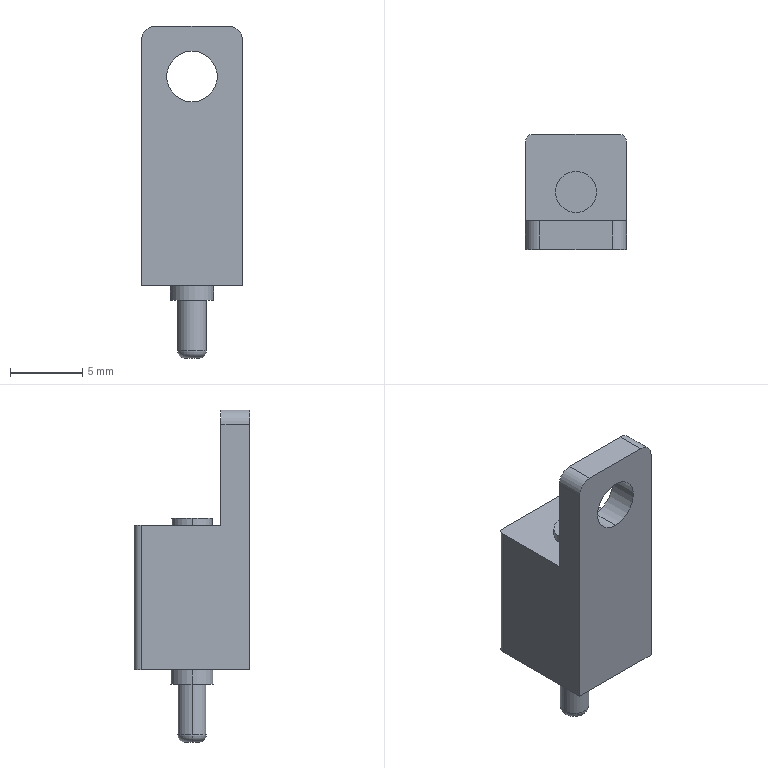Part | SolidWorks | features ICE 5, Fillet 3, Extrusion 1 | 1 solid | 25 faces | box 7 x 8 x 23 mm | volume 673.267 mm3 | cylinder 12 | plane 11 | torus 2 | commonest cylinder face diameters 2 x4 1 x2 2.853 x2 2.98 x2 3.5 x2
STEP:
#1=CARTESIAN_POINT('',(0.,-4.,12.75));
#2=VERTEX_POINT('',#1);
#3=CARTESIAN_POINT('',(0.,-4.,16.25));
#4=VERTEX_POINT('',#3);
#5=CARTESIAN_POINT('',(0.,-4.,14.5));
#6=DIRECTION('',(0.,1.,0.));
#7=DIRECTION('',(0.,0.,1.));
#8=AXIS2_PLACEMENT_3D('',#5,#6,#7);
#9=CIRCLE('',#8,1.75);
#10=EDGE_CURVE('',#2,#4,#9,.T.);
#11=ORIENTED_EDGE('',*,*,#10,.F.);
#12=CARTESIAN_POINT('',(0.,-2.,12.75));
#13=VERTEX_POINT('',#12);
#14=CARTESIAN_POINT('',(0.,-4.,12.75));
#15=DIRECTION('',(0.,1.,0.));
#16=VECTOR('',#15,1000.);
#17=LINE('',#14,#16);
#18=EDGE_CURVE('',#2,#13,#17,.T.);
#19=ORIENTED_EDGE('',*,*,#18,.T.);
#20=CARTESIAN_POINT('',(0.,-2.,16.25));
#21=VERTEX_POINT('',#20);
#22=CARTESIAN_POINT('',(0.,-2.,14.5));
#23=DIRECTION('',(0.,1.,0.));
#24=DIRECTION('',(0.,0.,1.));
#25=AXIS2_PLACEMENT_3D('',#22,#23,#24);
#26=CIRCLE('',#25,1.75);
#27=EDGE_CURVE('',#13,#21,#26,.T.);
#28=ORIENTED_EDGE('',*,*,#27,.T.);
#29=CARTESIAN_POINT('',(0.,-4.,16.25));
#30=DIRECTION('',(0.,1.,0.));
#31=VECTOR('',#30,1000.);
#32=LINE('',#29,#31);
#33=EDGE_CURVE('',#4,#21,#32,.T.);
#34=ORIENTED_EDGE('',*,*,#33,.F.);
#35=EDGE_LOOP('',(#11,#19,#28,#34));
#36=FACE_OUTER_BOUND('',#35,.T.);
#37=CARTESIAN_POINT('',(0.,-4.,14.5));
#38=DIRECTION('',(0.,1.,0.));
#39=DIRECTION('',(0.,0.,1.));
#40=AXIS2_PLACEMENT_3D('',#37,#38,#39);
#41=CYLINDRICAL_SURFACE('',#40,1.75);
#42=ADVANCED_FACE('',(#36),#41,.F.);
#43=CARTESIAN_POINT('',(1.427,0.,10.5));
#44=VERTEX_POINT('',#43);
#45=CARTESIAN_POINT('',(-1.427,0.,10.5));
#46=VERTEX_POINT('',#45);
#47=CARTESIAN_POINT('',(0.,0.,10.5));
#48=DIRECTION('',(0.,0.,1.));
#49=DIRECTION('',(1.,0.,0.));
#50=AXIS2_PLACEMENT_3D('',#47,#48,#49);
#51=CIRCLE('',#50,1.427);
#52=EDGE_CURVE('',#44,#46,#51,.T.);
#53=ORIENTED_EDGE('',*,*,#52,.F.);
#54=CARTESIAN_POINT('',(1.427,0.,10.));
#55=VERTEX_POINT('',#54);
#56=CARTESIAN_POINT('',(1.427,0.,10.5));
#57=DIRECTION('',(0.,0.,-1.));
#58=VECTOR('',#57,1000.);
#59=LINE('',#56,#58);
#60=EDGE_CURVE('',#44,#55,#59,.T.);
#61=ORIENTED_EDGE('',*,*,#60,.T.);
#62=CARTESIAN_POINT('',(-1.427,0.,10.));
#63=VERTEX_POINT('',#62);
#64=CARTESIAN_POINT('',(0.,0.,10.));
#65=DIRECTION('',(0.,0.,1.));
#66=DIRECTION('',(1.,0.,0.));
#67=AXIS2_PLACEMENT_3D('',#64,#65,#66);
#68=CIRCLE('',#67,1.427);
#69=EDGE_CURVE('',#55,#63,#68,.T.);
#70=ORIENTED_EDGE('',*,*,#69,.T.);
#71=CARTESIAN_POINT('',(-1.427,0.,10.5));
#72=DIRECTION('',(0.,0.,-1.));
#73=VECTOR('',#72,1000.);
#74=LINE('',#71,#73);
#75=EDGE_CURVE('',#46,#63,#74,.T.);
#76=ORIENTED_EDGE('',*,*,#75,.F.);
#77=EDGE_LOOP('',(#53,#61,#70,#76));
#78=FACE_OUTER_BOUND('',#77,.T.);
#79=CARTESIAN_POINT('',(0.,0.,10.5));
#80=DIRECTION('',(0.,0.,-1.));
#81=DIRECTION('',(-1.,0.,0.));
#82=AXIS2_PLACEMENT_3D('',#79,#80,#81);
#83=CYLINDRICAL_SURFACE('',#82,1.427);
#84=ADVANCED_FACE('',(#78),#83,.T.);
#85=CARTESIAN_POINT('',(1.,0.,-4.5));
#86=VERTEX_POINT('',#85);
#87=CARTESIAN_POINT('',(-1.,0.,-4.5));
#88=VERTEX_POINT('',#87);
#89=CARTESIAN_POINT('',(0.,0.,-4.5));
#90=DIRECTION('',(0.,0.,1.));
#91=DIRECTION('',(-1.,0.,0.));
#92=AXIS2_PLACEMENT_3D('',#89,#90,#91);
#93=CIRCLE('',#92,1.);
#94=EDGE_CURVE('',#86,#88,#93,.T.);
#95=ORIENTED_EDGE('',*,*,#94,.T.);
#96=CARTESIAN_POINT('',(-1.,0.,-1.));
#97=VERTEX_POINT('',#96);
#98=CARTESIAN_POINT('',(-1.,0.,-5.));
#99=DIRECTION('',(0.,0.,1.));
#100=VECTOR('',#99,1000.);
#101=LINE('',#98,#100);
#102=EDGE_CURVE('',#88,#97,#101,.T.);
#103=ORIENTED_EDGE('',*,*,#102,.T.);
#104=CARTESIAN_POINT('',(1.,0.,-1.));
#105=VERTEX_POINT('',#104);
#106=CARTESIAN_POINT('',(0.,0.,-1.));
#107=DIRECTION('',(0.,0.,-1.));
#108=DIRECTION('',(-1.,0.,0.));
#109=AXIS2_PLACEMENT_3D('',#106,#107,#108);
#110=CIRCLE('',#109,1.);
#111=EDGE_CURVE('',#97,#105,#110,.T.);
#112=ORIENTED_EDGE('',*,*,#111,.T.);
#113=CARTESIAN_POINT('',(1.,0.,-5.));
#114=DIRECTION('',(0.,0.,1.));
#115=VECTOR('',#114,1000.);
#116=LINE('',#113,#115);
#117=EDGE_CURVE('',#86,#105,#116,.T.);
#118=ORIENTED_EDGE('',*,*,#117,.F.);
#119=EDGE_LOOP('',(#95,#103,#112,#118));
#120=FACE_OUTER_BOUND('',#119,.T.);
#121=CARTESIAN_POINT('',(0.,0.,-5.));
#122=DIRECTION('',(0.,0.,1.));
#123=DIRECTION('',(1.,0.,0.));
#124=AXIS2_PLACEMENT_3D('',#121,#122,#123);
#125=CYLINDRICAL_SURFACE('',#124,1.);
#126=ADVANCED_FACE('',(#120),#125,.T.);
#127=ORIENTED_EDGE('',*,*,#94,.F.);
#128=CARTESIAN_POINT('',(0.5,0.,-5.));
#129=VERTEX_POINT('',#128);
#130=CARTESIAN_POINT('',(0.5,0.,-4.5));
#131=DIRECTION('',(0.,1.,0.));
#132=DIRECTION('',(-1.,0.,0.));
#133=AXIS2_PLACEMENT_3D('',#130,#131,#132);
#134=CIRCLE('',#133,0.5);
#135=EDGE_CURVE('',#86,#129,#134,.T.);
#136=ORIENTED_EDGE('',*,*,#135,.T.);
#137=CARTESIAN_POINT('',(-0.5,0.,-5.));
#138=VERTEX_POINT('',#137);
#139=CARTESIAN_POINT('',(0.,0.,-5.));
#140=DIRECTION('',(0.,0.,-1.));
#141=DIRECTION('',(-1.,0.,0.));
#142=AXIS2_PLACEMENT_3D('',#139,#140,#141);
#143=CIRCLE('',#142,0.5);
#144=EDGE_CURVE('',#138,#129,#143,.T.);
#145=ORIENTED_EDGE('',*,*,#144,.F.);
#146=CARTESIAN_POINT('',(-0.5,0.,-4.5));
#147=DIRECTION('',(0.,-1.,0.));
#148=DIRECTION('',(0.,0.,-1.));
#149=AXIS2_PLACEMENT_3D('',#146,#147,#148);
#150=CIRCLE('',#149,0.5);
#151=EDGE_CURVE('',#88,#138,#150,.T.);
#152=ORIENTED_EDGE('',*,*,#151,.F.);
#153=EDGE_LOOP('',(#127,#136,#145,#152));
#154=FACE_OUTER_BOUND('',#153,.T.);
#155=CARTESIAN_POINT('',(0.,0.,-4.5));
#156=DIRECTION('',(0.,0.,-1.));
#157=DIRECTION('',(-1.,0.,0.));
#158=AXIS2_PLACEMENT_3D('',#155,#156,#157);
#159=TOROIDAL_SURFACE('',#158,0.5,0.5);
#160=ADVANCED_FACE('',(#154),#159,.T.);
#161=CARTESIAN_POINT('',(-1.49,0.,-1.));
#162=VERTEX_POINT('',#161);
#163=CARTESIAN_POINT('',(1.49,0.,-1.));
#164=VERTEX_POINT('',#163);
#165=CARTESIAN_POINT('',(0.,0.,-1.));
#166=DIRECTION('',(0.,0.,-1.));
#167=DIRECTION('',(-1.,0.,0.));
#168=AXIS2_PLACEMENT_3D('',#165,#166,#167);
#169=CIRCLE('',#168,1.49);
#170=EDGE_CURVE('',#162,#164,#169,.T.);
#171=ORIENTED_EDGE('',*,*,#170,.F.);
#172=CARTESIAN_POINT('',(-1.49,0.,0.));
#173=VERTEX_POINT('',#172);
#174=CARTESIAN_POINT('',(-1.49,0.,-1.));
#175=DIRECTION('',(0.,0.,1.));
#176=VECTOR('',#175,1000.);
#177=LINE('',#174,#176);
#178=EDGE_CURVE('',#162,#173,#177,.T.);
#179=ORIENTED_EDGE('',*,*,#178,.T.);
#180=CARTESIAN_POINT('',(1.49,0.,0.));
#181=VERTEX_POINT('',#180);
#182=CARTESIAN_POINT('',(0.,0.,0.));
#183=DIRECTION('',(0.,0.,-1.));
#184=DIRECTION('',(1.,0.,0.));
#185=AXIS2_PLACEMENT_3D('',#182,#183,#184);
#186=CIRCLE('',#185,1.49);
#187=EDGE_CURVE('',#173,#181,#186,.T.);
#188=ORIENTED_EDGE('',*,*,#187,.T.);
#189=CARTESIAN_POINT('',(1.49,0.,-1.));
#190=DIRECTION('',(0.,0.,1.));
#191=VECTOR('',#190,1000.);
#192=LINE('',#189,#191);
#193=EDGE_CURVE('',#164,#181,#192,.T.);
#194=ORIENTED_EDGE('',*,*,#193,.F.);
#195=EDGE_LOOP('',(#171,#179,#188,#194));
#196=FACE_OUTER_BOUND('',#195,.T.);
#197=CARTESIAN_POINT('',(0.,0.,-1.));
#198=DIRECTION('',(0.,0.,1.));
#199=DIRECTION('',(1.,0.,0.));
#200=AXIS2_PLACEMENT_3D('',#197,#198,#199);
#201=CYLINDRICAL_SURFACE('',#200,1.49);
#202=ADVANCED_FACE('',(#196),#201,.T.);
#203=CARTESIAN_POINT('',(3.5,-2.,17.));
#204=VERTEX_POINT('',#203);
#205=CARTESIAN_POINT('',(3.5,-2.,10.));
#206=VERTEX_POINT('',#205);
#207=CARTESIAN_POINT('',(3.5,-2.,18.));
#208=DIRECTION('',(0.,0.,-1.));
#209=VECTOR('',#208,1000.);
#210=LINE('',#207,#209);
#211=EDGE_CURVE('',#204,#206,#210,.T.);
#212=ORIENTED_EDGE('',*,*,#211,.F.);
#213=CARTESIAN_POINT('',(3.5,-4.,17.));
#214=VERTEX_POINT('',#213);
#215=CARTESIAN_POINT('',(3.5,-4.,17.));
#216=DIRECTION('',(0.,-1.,0.));
#217=VECTOR('',#216,1000.);
#218=LINE('',#215,#217);
#219=EDGE_CURVE('',#204,#214,#218,.T.);
#220=ORIENTED_EDGE('',*,*,#219,.T.);
#221=CARTESIAN_POINT('',(3.5,-4.,0.));
#222=VERTEX_POINT('',#221);
#223=CARTESIAN_POINT('',(3.5,-4.,10.));
#224=DIRECTION('',(0.,0.,-1.));
#225=VECTOR('',#224,1000.);
#226=LINE('',#223,#225);
#227=EDGE_CURVE('',#214,#222,#226,.T.);
#228=ORIENTED_EDGE('',*,*,#227,.T.);
#229=CARTESIAN_POINT('',(3.5,3.5,0.));
#230=VERTEX_POINT('',#229);
#231=CARTESIAN_POINT('',(3.5,4.,0.));
#232=DIRECTION('',(0.,1.,0.));
#233=VECTOR('',#232,1000.);
#234=LINE('',#231,#233);
#235=EDGE_CURVE('',#222,#230,#234,.T.);
#236=ORIENTED_EDGE('',*,*,#235,.T.);
#237=CARTESIAN_POINT('',(3.5,3.5,10.));
#238=VERTEX_POINT('',#237);
#239=CARTESIAN_POINT('',(3.5,3.5,10.));
#240=DIRECTION('',(0.,0.,1.));
#241=VECTOR('',#240,1000.);
#242=LINE('',#239,#241);
#243=EDGE_CURVE('',#230,#238,#242,.T.);
#244=ORIENTED_EDGE('',*,*,#243,.T.);
#245=CARTESIAN_POINT('',(3.5,4.,10.));
#246=DIRECTION('',(0.,1.,0.));
#247=VECTOR('',#246,1000.);
#248=LINE('',#245,#247);
#249=EDGE_CURVE('',#206,#238,#248,.T.);
#250=ORIENTED_EDGE('',*,*,#249,.F.);
#251=EDGE_LOOP('',(#212,#220,#228,#236,#244,#250));
#252=FACE_OUTER_BOUND('',#251,.T.);
#253=CARTESIAN_POINT('',(3.5,4.,10.));
#254=DIRECTION('',(-1.,0.,0.));
#255=DIRECTION('',(0.,-1.,0.));
#256=AXIS2_PLACEMENT_3D('',#253,#254,#255);
#257=PLANE('',#256);
#258=ADVANCED_FACE('',(#252),#257,.F.);
#259=CARTESIAN_POINT('',(3.,4.,0.));
#260=VERTEX_POINT('',#259);
#261=CARTESIAN_POINT('',(-3.,4.,0.));
#262=VERTEX_POINT('',#261);
#263=CARTESIAN_POINT('',(-3.5,4.,0.));
#264=DIRECTION('',(-1.,0.,0.));
#265=VECTOR('',#264,1000.);
#266=LINE('',#263,#265);
#267=EDGE_CURVE('',#260,#262,#266,.T.);
#268=ORIENTED_EDGE('',*,*,#267,.T.);
#269=CARTESIAN_POINT('',(-3.,4.,10.));
#270=VERTEX_POINT('',#269);
#271=CARTESIAN_POINT('',(-3.,4.,10.));
#272=DIRECTION('',(0.,0.,1.));
#273=VECTOR('',#272,1000.);
#274=LINE('',#271,#273);
#275=EDGE_CURVE('',#262,#270,#274,.T.);
#276=ORIENTED_EDGE('',*,*,#275,.T.);
#277=CARTESIAN_POINT('',(3.,4.,10.));
#278=VERTEX_POINT('',#277);
#279=CARTESIAN_POINT('',(-3.5,4.,10.));
#280=DIRECTION('',(-1.,0.,0.));
#281=VECTOR('',#280,1000.);
#282=LINE('',#279,#281);
#283=EDGE_CURVE('',#278,#270,#282,.T.);
#284=ORIENTED_EDGE('',*,*,#283,.F.);
#285=CARTESIAN_POINT('',(3.,4.,10.));
#286=DIRECTION('',(0.,0.,-1.));
#287=VECTOR('',#286,1000.);
#288=LINE('',#285,#287);
#289=EDGE_CURVE('',#278,#260,#288,.T.);
#290=ORIENTED_EDGE('',*,*,#289,.T.);
#291=EDGE_LOOP('',(#268,#276,#284,#290));
#292=FACE_OUTER_BOUND('',#291,.T.);
#293=CARTESIAN_POINT('',(-3.5,4.,10.));
#294=DIRECTION('',(0.,-1.,0.));
#295=DIRECTION('',(0.,0.,-1.));
#296=AXIS2_PLACEMENT_3D('',#293,#294,#295);
#297=PLANE('',#296);
#298=ADVANCED_FACE('',(#292),#297,.F.);
#299=CARTESIAN_POINT('',(-3.5,-4.,17.));
#300=VERTEX_POINT('',#299);
#301=CARTESIAN_POINT('',(-3.5,-4.,0.));
#302=VERTEX_POINT('',#301);
#303=CARTESIAN_POINT('',(-3.5,-4.,10.));
#304=DIRECTION('',(0.,0.,-1.));
#305=VECTOR('',#304,1000.);
#306=LINE('',#303,#305);
#307=EDGE_CURVE('',#300,#302,#306,.T.);
#308=ORIENTED_EDGE('',*,*,#307,.F.);
#309=CARTESIAN_POINT('',(-3.5,-2.,17.));
#310=VERTEX_POINT('',#309);
#311=CARTESIAN_POINT('',(-3.5,-2.,17.));
#312=DIRECTION('',(0.,1.,0.));
#313=VECTOR('',#312,1000.);
#314=LINE('',#311,#313);
#315=EDGE_CURVE('',#300,#310,#314,.T.);
#316=ORIENTED_EDGE('',*,*,#315,.T.);
#317=CARTESIAN_POINT('',(-3.5,-2.,10.));
#318=VERTEX_POINT('',#317);
#319=CARTESIAN_POINT('',(-3.5,-2.,18.));
#320=DIRECTION('',(0.,0.,-1.));
#321=VECTOR('',#320,1000.);
#322=LINE('',#319,#321);
#323=EDGE_CURVE('',#310,#318,#322,.T.);
#324=ORIENTED_EDGE('',*,*,#323,.T.);
#325=CARTESIAN_POINT('',(-3.5,3.5,10.));
#326=VERTEX_POINT('',#325);
#327=CARTESIAN_POINT('',(-3.5,4.,10.));
#328=DIRECTION('',(0.,-1.,0.));
#329=VECTOR('',#328,1000.);
#330=LINE('',#327,#329);
#331=EDGE_CURVE('',#326,#318,#330,.T.);
#332=ORIENTED_EDGE('',*,*,#331,.F.);
#333=CARTESIAN_POINT('',(-3.5,3.5,0.));
#334=VERTEX_POINT('',#333);
#335=CARTESIAN_POINT('',(-3.5,3.5,10.));
#336=DIRECTION('',(0.,0.,-1.));
#337=VECTOR('',#336,1000.);
#338=LINE('',#335,#337);
#339=EDGE_CURVE('',#326,#334,#338,.T.);
#340=ORIENTED_EDGE('',*,*,#339,.T.);
#341=CARTESIAN_POINT('',(-3.5,4.,0.));
#342=DIRECTION('',(0.,-1.,0.));
#343=VECTOR('',#342,1000.);
#344=LINE('',#341,#343);
#345=EDGE_CURVE('',#334,#302,#344,.T.);
#346=ORIENTED_EDGE('',*,*,#345,.T.);
#347=EDGE_LOOP('',(#308,#316,#324,#332,#340,#346));
#348=FACE_OUTER_BOUND('',#347,.T.);
#349=CARTESIAN_POINT('',(-3.5,4.,10.));
#350=DIRECTION('',(1.,0.,0.));
#351=DIRECTION('',(0.,1.,0.));
#352=AXIS2_PLACEMENT_3D('',#349,#350,#351);
#353=PLANE('',#352);
#354=ADVANCED_FACE('',(#348),#353,.F.);
#355=CARTESIAN_POINT('',(0.,-4.,14.5));
#356=DIRECTION('',(0.,1.,0.));
#357=DIRECTION('',(0.,0.,1.));
#358=AXIS2_PLACEMENT_3D('',#355,#356,#357);
#359=CIRCLE('',#358,1.75);
#360=EDGE_CURVE('',#4,#2,#359,.T.);
#361=ORIENTED_EDGE('',*,*,#360,.T.);
#362=ORIENTED_EDGE('',*,*,#10,.T.);
#363=EDGE_LOOP('',(#361,#362));
#364=FACE_BOUND('',#363,.T.);
#365=CARTESIAN_POINT('',(-2.5,-4.,18.));
#366=VERTEX_POINT('',#365);
#367=CARTESIAN_POINT('',(2.5,-4.,18.));
#368=VERTEX_POINT('',#367);
#369=CARTESIAN_POINT('',(-3.5,-4.,18.));
#370=DIRECTION('',(1.,0.,0.));
#371=VECTOR('',#370,1000.);
#372=LINE('',#369,#371);
#373=EDGE_CURVE('',#366,#368,#372,.T.);
#374=ORIENTED_EDGE('',*,*,#373,.F.);
#375=CARTESIAN_POINT('',(-2.5,-4.,17.));
#376=DIRECTION('',(0.,-1.,0.));
#377=DIRECTION('',(0.,0.,1.));
#378=AXIS2_PLACEMENT_3D('',#375,#376,#377);
#379=CIRCLE('',#378,1.);
#380=EDGE_CURVE('',#366,#300,#379,.T.);
#381=ORIENTED_EDGE('',*,*,#380,.T.);
#382=ORIENTED_EDGE('',*,*,#307,.T.);
#383=CARTESIAN_POINT('',(-3.5,-4.,0.));
#384=DIRECTION('',(1.,0.,0.));
#385=VECTOR('',#384,1000.);
#386=LINE('',#383,#385);
#387=EDGE_CURVE('',#302,#222,#386,.T.);
#388=ORIENTED_EDGE('',*,*,#387,.T.);
#389=ORIENTED_EDGE('',*,*,#227,.F.);
#390=CARTESIAN_POINT('',(2.5,-4.,17.));
#391=DIRECTION('',(0.,-1.,0.));
#392=DIRECTION('',(0.,0.,1.));
#393=AXIS2_PLACEMENT_3D('',#390,#391,#392);
#394=CIRCLE('',#393,1.);
#395=EDGE_CURVE('',#214,#368,#394,.T.);
#396=ORIENTED_EDGE('',*,*,#395,.T.);
#397=EDGE_LOOP('',(#374,#381,#382,#388,#389,#396));
#398=FACE_OUTER_BOUND('',#397,.T.);
#399=CARTESIAN_POINT('',(-3.5,-4.,10.));
#400=DIRECTION('',(0.,1.,0.));
#401=DIRECTION('',(0.,0.,1.));
#402=AXIS2_PLACEMENT_3D('',#399,#400,#401);
#403=PLANE('',#402);
#404=ADVANCED_FACE('',(#364,#398),#403,.F.);
#405=CARTESIAN_POINT('',(0.,0.,10.));
#406=DIRECTION('',(0.,0.,1.));
#407=DIRECTION('',(1.,0.,0.));
#408=AXIS2_PLACEMENT_3D('',#405,#406,#407);
#409=CIRCLE('',#408,1.427);
#410=EDGE_CURVE('',#63,#55,#409,.T.);
#411=ORIENTED_EDGE('',*,*,#410,.F.);
#412=ORIENTED_EDGE('',*,*,#69,.F.);
#413=EDGE_LOOP('',(#411,#412));
#414=FACE_BOUND('',#413,.T.);
#415=ORIENTED_EDGE('',*,*,#283,.T.);
#416=CARTESIAN_POINT('',(-3.,3.5,10.));
#417=DIRECTION('',(0.,0.,1.));
#418=DIRECTION('',(1.,0.,0.));
#419=AXIS2_PLACEMENT_3D('',#416,#417,#418);
#420=CIRCLE('',#419,0.5);
#421=EDGE_CURVE('',#270,#326,#420,.T.);
#422=ORIENTED_EDGE('',*,*,#421,.T.);
#423=ORIENTED_EDGE('',*,*,#331,.T.);
#424=CARTESIAN_POINT('',(-3.5,-2.,10.));
#425=DIRECTION('',(-1.,0.,0.));
#426=VECTOR('',#425,1000.);
#427=LINE('',#424,#426);
#428=EDGE_CURVE('',#206,#318,#427,.T.);
#429=ORIENTED_EDGE('',*,*,#428,.F.);
#430=ORIENTED_EDGE('',*,*,#249,.T.);
#431=CARTESIAN_POINT('',(3.,3.5,10.));
#432=DIRECTION('',(0.,0.,1.));
#433=DIRECTION('',(1.,0.,0.));
#434=AXIS2_PLACEMENT_3D('',#431,#432,#433);
#435=CIRCLE('',#434,0.5);
#436=EDGE_CURVE('',#238,#278,#435,.T.);
#437=ORIENTED_EDGE('',*,*,#436,.T.);
#438=EDGE_LOOP('',(#415,#422,#423,#429,#430,#437));
#439=FACE_OUTER_BOUND('',#438,.T.);
#440=CARTESIAN_POINT('',(0.,0.,10.));
#441=DIRECTION('',(0.,0.,1.));
#442=DIRECTION('',(1.,0.,0.));
#443=AXIS2_PLACEMENT_3D('',#440,#441,#442);
#444=PLANE('',#443);
#445=ADVANCED_FACE('',(#414,#439),#444,.T.);
#446=CARTESIAN_POINT('',(0.,0.,0.));
#447=DIRECTION('',(0.,0.,-1.));
#448=DIRECTION('',(1.,0.,0.));
#449=AXIS2_PLACEMENT_3D('',#446,#447,#448);
#450=CIRCLE('',#449,1.49);
#451=EDGE_CURVE('',#181,#173,#450,.T.);
#452=ORIENTED_EDGE('',*,*,#451,.F.);
#453=ORIENTED_EDGE('',*,*,#187,.F.);
#454=EDGE_LOOP('',(#452,#453));
#455=FACE_BOUND('',#454,.T.);
#456=ORIENTED_EDGE('',*,*,#345,.F.);
#457=CARTESIAN_POINT('',(-3.,3.5,0.));
#458=DIRECTION('',(0.,0.,-1.));
#459=DIRECTION('',(1.,0.,0.));
#460=AXIS2_PLACEMENT_3D('',#457,#458,#459);
#461=CIRCLE('',#460,0.5);
#462=EDGE_CURVE('',#334,#262,#461,.T.);
#463=ORIENTED_EDGE('',*,*,#462,.T.);
#464=ORIENTED_EDGE('',*,*,#267,.F.);
#465=CARTESIAN_POINT('',(3.,3.5,0.));
#466=DIRECTION('',(0.,0.,-1.));
#467=DIRECTION('',(1.,0.,0.));
#468=AXIS2_PLACEMENT_3D('',#465,#466,#467);
#469=CIRCLE('',#468,0.5);
#470=EDGE_CURVE('',#260,#230,#469,.T.);
#471=ORIENTED_EDGE('',*,*,#470,.T.);
#472=ORIENTED_EDGE('',*,*,#235,.F.);
#473=ORIENTED_EDGE('',*,*,#387,.F.);
#474=EDGE_LOOP('',(#456,#463,#464,#471,#472,#473));
#475=FACE_OUTER_BOUND('',#474,.T.);
#476=CARTESIAN_POINT('',(0.,0.,0.));
#477=DIRECTION('',(0.,0.,1.));
#478=DIRECTION('',(1.,0.,0.));
#479=AXIS2_PLACEMENT_3D('',#476,#477,#478);
#480=PLANE('',#479);
#481=ADVANCED_FACE('',(#455,#475),#480,.F.);
#482=CARTESIAN_POINT('',(0.,-2.,14.5));
#483=DIRECTION('',(0.,1.,0.));
#484=DIRECTION('',(0.,0.,1.));
#485=AXIS2_PLACEMENT_3D('',#482,#483,#484);
#486=CIRCLE('',#485,1.75);
#487=EDGE_CURVE('',#21,#13,#486,.T.);
#488=ORIENTED_EDGE('',*,*,#487,.F.);
#489=ORIENTED_EDGE('',*,*,#27,.F.);
#490=EDGE_LOOP('',(#488,#489));
#491=FACE_BOUND('',#490,.T.);
#492=ORIENTED_EDGE('',*,*,#323,.F.);
#493=CARTESIAN_POINT('',(-2.5,-2.,18.));
#494=VERTEX_POINT('',#493);
#495=CARTESIAN_POINT('',(-2.5,-2.,17.));
#496=DIRECTION('',(0.,1.,0.));
#497=DIRECTION('',(0.,0.,-1.));
#498=AXIS2_PLACEMENT_3D('',#495,#496,#497);
#499=CIRCLE('',#498,1.);
#500=EDGE_CURVE('',#310,#494,#499,.T.);
#501=ORIENTED_EDGE('',*,*,#500,.T.);
#502=CARTESIAN_POINT('',(2.5,-2.,18.));
#503=VERTEX_POINT('',#502);
#504=CARTESIAN_POINT('',(-3.5,-2.,18.));
#505=DIRECTION('',(-1.,0.,0.));
#506=VECTOR('',#505,1000.);
#507=LINE('',#504,#506);
#508=EDGE_CURVE('',#503,#494,#507,.T.);
#509=ORIENTED_EDGE('',*,*,#508,.F.);
#510=CARTESIAN_POINT('',(2.5,-2.,17.));
#511=DIRECTION('',(0.,1.,0.));
#512=DIRECTION('',(0.,0.,-1.));
#513=AXIS2_PLACEMENT_3D('',#510,#511,#512);
#514=CIRCLE('',#513,1.);
#515=EDGE_CURVE('',#503,#204,#514,.T.);
#516=ORIENTED_EDGE('',*,*,#515,.T.);
#517=ORIENTED_EDGE('',*,*,#211,.T.);
#518=ORIENTED_EDGE('',*,*,#428,.T.);
#519=EDGE_LOOP('',(#492,#501,#509,#516,#517,#518));
#520=FACE_OUTER_BOUND('',#519,.T.);
#521=CARTESIAN_POINT('',(-3.5,-2.,18.));
#522=DIRECTION('',(0.,-1.,0.));
#523=DIRECTION('',(0.,0.,-1.));
#524=AXIS2_PLACEMENT_3D('',#521,#522,#523);
#525=PLANE('',#524);
#526=ADVANCED_FACE('',(#491,#520),#525,.F.);
#527=ORIENTED_EDGE('',*,*,#508,.T.);
#528=CARTESIAN_POINT('',(-2.5,-4.,18.));
#529=DIRECTION('',(0.,-1.,0.));
#530=VECTOR('',#529,1000.);
#531=LINE('',#528,#530);
#532=EDGE_CURVE('',#494,#366,#531,.T.);
#533=ORIENTED_EDGE('',*,*,#532,.T.);
#534=ORIENTED_EDGE('',*,*,#373,.T.);
#535=CARTESIAN_POINT('',(2.5,-2.,18.));
#536=DIRECTION('',(0.,1.,0.));
#537=VECTOR('',#536,1000.);
#538=LINE('',#535,#537);
#539=EDGE_CURVE('',#368,#503,#538,.T.);
#540=ORIENTED_EDGE('',*,*,#539,.T.);
#541=EDGE_LOOP('',(#527,#533,#534,#540));
#542=FACE_OUTER_BOUND('',#541,.T.);
#543=CARTESIAN_POINT('',(0.,0.,18.));
#544=DIRECTION('',(0.,0.,1.));
#545=DIRECTION('',(1.,0.,0.));
#546=AXIS2_PLACEMENT_3D('',#543,#544,#545);
#547=PLANE('',#546);
#548=ADVANCED_FACE('',(#542),#547,.T.);
#549=ORIENTED_EDGE('',*,*,#178,.F.);
#550=CARTESIAN_POINT('',(0.,0.,-1.));
#551=DIRECTION('',(0.,0.,-1.));
#552=DIRECTION('',(-1.,0.,0.));
#553=AXIS2_PLACEMENT_3D('',#550,#551,#552);
#554=CIRCLE('',#553,1.49);
#555=EDGE_CURVE('',#164,#162,#554,.T.);
#556=ORIENTED_EDGE('',*,*,#555,.F.);
#557=ORIENTED_EDGE('',*,*,#193,.T.);
#558=ORIENTED_EDGE('',*,*,#451,.T.);
#559=EDGE_LOOP('',(#549,#556,#557,#558));
#560=FACE_OUTER_BOUND('',#559,.T.);
#561=CARTESIAN_POINT('',(0.,0.,-1.));
#562=DIRECTION('',(0.,0.,1.));
#563=DIRECTION('',(1.,0.,0.));
#564=AXIS2_PLACEMENT_3D('',#561,#562,#563);
#565=CYLINDRICAL_SURFACE('',#564,1.49);
#566=ADVANCED_FACE('',(#560),#565,.T.);
#567=CARTESIAN_POINT('',(0.,0.,-1.));
#568=DIRECTION('',(0.,0.,-1.));
#569=DIRECTION('',(-1.,0.,0.));
#570=AXIS2_PLACEMENT_3D('',#567,#568,#569);
#571=CIRCLE('',#570,1.);
#572=EDGE_CURVE('',#105,#97,#571,.T.);
#573=ORIENTED_EDGE('',*,*,#572,.F.);
#574=ORIENTED_EDGE('',*,*,#111,.F.);
#575=EDGE_LOOP('',(#573,#574));
#576=FACE_BOUND('',#575,.T.);
#577=ORIENTED_EDGE('',*,*,#555,.T.);
#578=ORIENTED_EDGE('',*,*,#170,.T.);
#579=EDGE_LOOP('',(#577,#578));
#580=FACE_OUTER_BOUND('',#579,.T.);
#581=CARTESIAN_POINT('',(0.,0.,-1.));
#582=DIRECTION('',(0.,0.,-1.));
#583=DIRECTION('',(-1.,0.,0.));
#584=AXIS2_PLACEMENT_3D('',#581,#582,#583);
#585=PLANE('',#584);
#586=ADVANCED_FACE('',(#576,#580),#585,.T.);
#587=ORIENTED_EDGE('',*,*,#144,.T.);
#588=CARTESIAN_POINT('',(0.,0.,-5.));
#589=DIRECTION('',(0.,0.,-1.));
#590=DIRECTION('',(-1.,0.,0.));
#591=AXIS2_PLACEMENT_3D('',#588,#589,#590);
#592=CIRCLE('',#591,0.5);
#593=EDGE_CURVE('',#129,#138,#592,.T.);
#594=ORIENTED_EDGE('',*,*,#593,.T.);
#595=EDGE_LOOP('',(#587,#594));
#596=FACE_OUTER_BOUND('',#595,.T.);
#597=CARTESIAN_POINT('',(0.,0.,-5.));
#598=DIRECTION('',(0.,0.,-1.));
#599=DIRECTION('',(-1.,0.,0.));
#600=AXIS2_PLACEMENT_3D('',#597,#598,#599);
#601=PLANE('',#600);
#602=ADVANCED_FACE('',(#596),#601,.T.);
#603=ORIENTED_EDGE('',*,*,#135,.F.);
#604=CARTESIAN_POINT('',(0.,0.,-4.5));
#605=DIRECTION('',(0.,0.,1.));
#606=DIRECTION('',(-1.,0.,0.));
#607=AXIS2_PLACEMENT_3D('',#604,#605,#606);
#608=CIRCLE('',#607,1.);
#609=EDGE_CURVE('',#88,#86,#608,.T.);
#610=ORIENTED_EDGE('',*,*,#609,.F.);
#611=ORIENTED_EDGE('',*,*,#151,.T.);
#612=ORIENTED_EDGE('',*,*,#593,.F.);
#613=EDGE_LOOP('',(#603,#610,#611,#612));
#614=FACE_OUTER_BOUND('',#613,.T.);
#615=CARTESIAN_POINT('',(0.,0.,-4.5));
#616=DIRECTION('',(0.,0.,-1.));
#617=DIRECTION('',(-1.,0.,0.));
#618=AXIS2_PLACEMENT_3D('',#615,#616,#617);
#619=TOROIDAL_SURFACE('',#618,0.5,0.5);
#620=ADVANCED_FACE('',(#614),#619,.T.);
#621=ORIENTED_EDGE('',*,*,#102,.F.);
#622=ORIENTED_EDGE('',*,*,#609,.T.);
#623=ORIENTED_EDGE('',*,*,#117,.T.);
#624=ORIENTED_EDGE('',*,*,#572,.T.);
#625=EDGE_LOOP('',(#621,#622,#623,#624));
#626=FACE_OUTER_BOUND('',#625,.T.);
#627=CARTESIAN_POINT('',(0.,0.,-5.));
#628=DIRECTION('',(0.,0.,1.));
#629=DIRECTION('',(1.,0.,0.));
#630=AXIS2_PLACEMENT_3D('',#627,#628,#629);
#631=CYLINDRICAL_SURFACE('',#630,1.);
#632=ADVANCED_FACE('',(#626),#631,.T.);
#633=ORIENTED_EDGE('',*,*,#60,.F.);
#634=CARTESIAN_POINT('',(0.,0.,10.5));
#635=DIRECTION('',(0.,0.,1.));
#636=DIRECTION('',(1.,0.,0.));
#637=AXIS2_PLACEMENT_3D('',#634,#635,#636);
#638=CIRCLE('',#637,1.427);
#639=EDGE_CURVE('',#46,#44,#638,.T.);
#640=ORIENTED_EDGE('',*,*,#639,.F.);
#641=ORIENTED_EDGE('',*,*,#75,.T.);
#642=ORIENTED_EDGE('',*,*,#410,.T.);
#643=EDGE_LOOP('',(#633,#640,#641,#642));
#644=FACE_OUTER_BOUND('',#643,.T.);
#645=CARTESIAN_POINT('',(0.,0.,10.5));
#646=DIRECTION('',(0.,0.,-1.));
#647=DIRECTION('',(-1.,0.,0.));
#648=AXIS2_PLACEMENT_3D('',#645,#646,#647);
#649=CYLINDRICAL_SURFACE('',#648,1.427);
#650=ADVANCED_FACE('',(#644),#649,.T.);
#651=ORIENTED_EDGE('',*,*,#639,.T.);
#652=ORIENTED_EDGE('',*,*,#52,.T.);
#653=EDGE_LOOP('',(#651,#652));
#654=FACE_OUTER_BOUND('',#653,.T.);
#655=CARTESIAN_POINT('',(0.,0.,10.5));
#656=DIRECTION('',(0.,0.,1.));
#657=DIRECTION('',(1.,0.,0.));
#658=AXIS2_PLACEMENT_3D('',#655,#656,#657);
#659=PLANE('',#658);
#660=ADVANCED_FACE('',(#654),#659,.T.);
#661=ORIENTED_EDGE('',*,*,#421,.F.);
#662=ORIENTED_EDGE('',*,*,#275,.F.);
#663=ORIENTED_EDGE('',*,*,#462,.F.);
#664=ORIENTED_EDGE('',*,*,#339,.F.);
#665=EDGE_LOOP('',(#661,#662,#663,#664));
#666=FACE_OUTER_BOUND('',#665,.T.);
#667=CARTESIAN_POINT('',(-3.,3.5,10.));
#668=DIRECTION('',(0.,0.,-1.));
#669=DIRECTION('',(-1.,0.,0.));
#670=AXIS2_PLACEMENT_3D('',#667,#668,#669);
#671=CYLINDRICAL_SURFACE('',#670,0.5);
#672=ADVANCED_FACE('',(#666),#671,.T.);
#673=ORIENTED_EDGE('',*,*,#436,.F.);
#674=ORIENTED_EDGE('',*,*,#243,.F.);
#675=ORIENTED_EDGE('',*,*,#470,.F.);
#676=ORIENTED_EDGE('',*,*,#289,.F.);
#677=EDGE_LOOP('',(#673,#674,#675,#676));
#678=FACE_OUTER_BOUND('',#677,.T.);
#679=CARTESIAN_POINT('',(3.,3.5,10.));
#680=DIRECTION('',(0.,0.,-1.));
#681=DIRECTION('',(-1.,0.,0.));
#682=AXIS2_PLACEMENT_3D('',#679,#680,#681);
#683=CYLINDRICAL_SURFACE('',#682,0.5);
#684=ADVANCED_FACE('',(#678),#683,.T.);
#685=ORIENTED_EDGE('',*,*,#500,.F.);
#686=ORIENTED_EDGE('',*,*,#315,.F.);
#687=ORIENTED_EDGE('',*,*,#380,.F.);
#688=ORIENTED_EDGE('',*,*,#532,.F.);
#689=EDGE_LOOP('',(#685,#686,#687,#688));
#690=FACE_OUTER_BOUND('',#689,.T.);
#691=CARTESIAN_POINT('',(-2.5,0.,17.));
#692=DIRECTION('',(0.,1.,0.));
#693=DIRECTION('',(-1.,0.,0.));
#694=AXIS2_PLACEMENT_3D('',#691,#692,#693);
#695=CYLINDRICAL_SURFACE('',#694,1.);
#696=ADVANCED_FACE('',(#690),#695,.T.);
#697=ORIENTED_EDGE('',*,*,#395,.F.);
#698=ORIENTED_EDGE('',*,*,#219,.F.);
#699=ORIENTED_EDGE('',*,*,#515,.F.);
#700=ORIENTED_EDGE('',*,*,#539,.F.);
#701=EDGE_LOOP('',(#697,#698,#699,#700));
#702=FACE_OUTER_BOUND('',#701,.T.);
#703=CARTESIAN_POINT('',(2.5,0.,17.));
#704=DIRECTION('',(0.,-1.,0.));
#705=DIRECTION('',(1.,0.,0.));
#706=AXIS2_PLACEMENT_3D('',#703,#704,#705);
#707=CYLINDRICAL_SURFACE('',#706,1.);
#708=ADVANCED_FACE('',(#702),#707,.T.);
#709=ORIENTED_EDGE('',*,*,#18,.F.);
#710=ORIENTED_EDGE('',*,*,#360,.F.);
#711=ORIENTED_EDGE('',*,*,#33,.T.);
#712=ORIENTED_EDGE('',*,*,#487,.T.);
#713=EDGE_LOOP('',(#709,#710,#711,#712));
#714=FACE_OUTER_BOUND('',#713,.T.);
#715=CARTESIAN_POINT('',(0.,-4.,14.5));
#716=DIRECTION('',(0.,1.,0.));
#717=DIRECTION('',(0.,0.,1.));
#718=AXIS2_PLACEMENT_3D('',#715,#716,#717);
#719=CYLINDRICAL_SURFACE('',#718,1.75);
#720=ADVANCED_FACE('',(#714),#719,.F.);
#721=CLOSED_SHELL('',(#42,#84,#126,#160,#202,#258,#298,#354,#404,#445,#481,#526,#548,#566,#586,#602,#620,#632,#650,#660,#672,#684,#696,#708,#720));
#722=MANIFOLD_SOLID_BREP('',#721);
#723=CARTESIAN_POINT('',(0.,0.,0.));
#724=DIRECTION('',(0.,0.,1.));
#725=DIRECTION('',(1.,0.,0.));
#726=AXIS2_PLACEMENT_3D('',#723,#724,#725);
#727=(LENGTH_UNIT()NAMED_UNIT(*)SI_UNIT(.MILLI.,.METRE.));
#728=UNCERTAINTY_MEASURE_WITH_UNIT(LENGTH_MEASURE(0.00001),#727,'','');
#729=(NAMED_UNIT(*)PLANE_ANGLE_UNIT()SI_UNIT($,.RADIAN.));
#730=(NAMED_UNIT(*)SI_UNIT($,.STERADIAN.)SOLID_ANGLE_UNIT());
#731=(GEOMETRIC_REPRESENTATION_CONTEXT(3)GLOBAL_UNCERTAINTY_ASSIGNED_CONTEXT((#728))GLOBAL_UNIT_ASSIGNED_CONTEXT((#727,#729,#730))REPRESENTATION_CONTEXT('',''));
#732=ADVANCED_BREP_SHAPE_REPRESENTATION('',(#722,#726),#731);